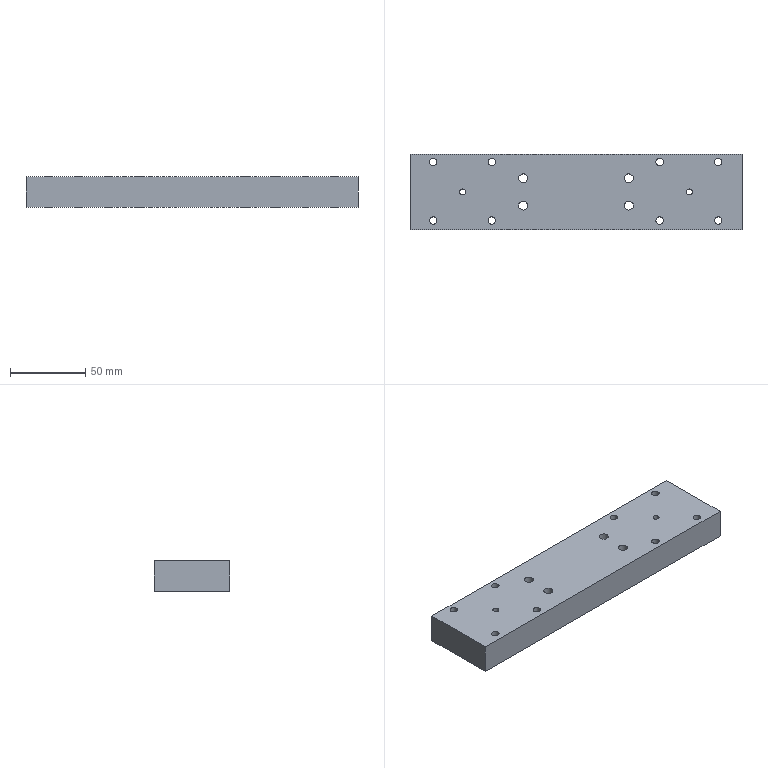NC program | NX | posted with a generic post | part box 220 x 50 x 20 mm
Whole program:
N10 G17 G21 G94 G90
(ZLEVEL_PROFILE_1 , TOOL : D10)
N12 T10 M6
N14 G54
N16 G17 G0 G90 X-42.544 Y30.1 S9500 M3
N18 G43 Z30. H10
N20 Z1.5
N22 G94 G1 X0. Z-0.73 F3000.
N24 X110.
N26 G2 X115.1 Y25. R5.1
N28 G1 Y-25.
N30 G2 X110. Y-30.1 R5.1
N32 G1 X-110.
N34 G2 X-115.1 Y-25. R5.1
N36 G1 Y25.
N38 G2 X-110. Y30.1 R5.1
N40 G1 X0.
N42 X41.8 Z-1.459
N44 X110.
N46 G2 X115.1 Y25. R5.1
N48 G1 Y-25.
N50 G2 X110. Y-30.1 R5.1
N52 G1 X-110.
N54 G2 X-115.1 Y-25. R5.1
N56 G1 Y25.
N58 G2 X-110. Y30.1 R5.1
N60 G1 X0.
N62 X41.8 Z-2.189
N64 X110.
N66 G2 X115.1 Y25. R5.1
N68 G1 Y-25.
N70 G2 X110. Y-30.1 R5.1
N72 G1 X-110.
N74 G2 X-115.1 Y-25. R5.1
N76 G1 Y25.
N78 G2 X-110. Y30.1 R5.1
N80 G1 X0.
N82 X41.8 Z-2.919
N84 X110.
N86 G2 X115.1 Y25. R5.1
N88 G1 Y-25.
N90 G2 X110. Y-30.1 R5.1
N92 G1 X-110.
N94 G2 X-115.1 Y-25. R5.1
N96 G1 Y25.
N98 G2 X-110. Y30.1 R5.1
N100 G1 X0.
N102 X41.8 Z-3.648
N104 X110.
N106 G2 X115.1 Y25. R5.1
N108 G1 Y-25.
N110 G2 X110. Y-30.1 R5.1
N112 G1 X-110.
N114 G2 X-115.1 Y-25. R5.1
N116 G1 Y25.
N118 G2 X-110. Y30.1 R5.1
N120 G1 X0.
N122 X41.8 Z-4.378
N124 X110.
N126 G2 X115.1 Y25. R5.1
N128 G1 Y-25.
N130 G2 X110. Y-30.1 R5.1
N132 G1 X-110.
N134 G2 X-115.1 Y-25. R5.1
N136 G1 Y25.
N138 G2 X-110. Y30.1 R5.1
N140 G1 X0.
N142 X41.8 Z-5.107
N144 X110.
N146 G2 X115.1 Y25. R5.1
N148 G1 Y-25.
N150 G2 X110. Y-30.1 R5.1
N152 G1 X-110.
N154 G2 X-115.1 Y-25. R5.1
N156 G1 Y25.
N158 G2 X-110. Y30.1 R5.1
N160 G1 X0.
N162 X41.8 Z-5.837
N164 X110.
N166 G2 X115.1 Y25. R5.1
N168 G1 Y-25.
N170 G2 X110. Y-30.1 R5.1
N172 G1 X-110.
N174 G2 X-115.1 Y-25. R5.1
N176 G1 Y25.
N178 G2 X-110. Y30.1 R5.1
N180 G1 X0.
N182 X41.8 Z-6.567
N184 X110.
N186 G2 X115.1 Y25. R5.1
N188 G1 Y-25.
N190 G2 X110. Y-30.1 R5.1
N192 G1 X-110.
N194 G2 X-115.1 Y-25. R5.1
N196 G1 Y25.
N198 G2 X-110. Y30.1 R5.1
N200 G1 X0.
N202 X41.8 Z-7.296
N204 X110.
N206 G2 X115.1 Y25. R5.1
N208 G1 Y-25.
N210 G2 X110. Y-30.1 R5.1
N212 G1 X-110.
N214 G2 X-115.1 Y-25. R5.1
N216 G1 Y25.
N218 G2 X-110. Y30.1 R5.1
N220 G1 X0.
N222 X41.8 Z-8.026
N224 X110.
N226 G2 X115.1 Y25. R5.1
N228 G1 Y-25.
N230 G2 X110. Y-30.1 R5.1
N232 G1 X-110.
N234 G2 X-115.1 Y-25. R5.1
N236 G1 Y25.
N238 G2 X-110. Y30.1 R5.1
N240 G1 X0.
N242 X41.8 Z-8.756
N244 X110.
N246 G2 X115.1 Y25. R5.1
N248 G1 Y-25.
N250 G2 X110. Y-30.1 R5.1
N252 G1 X-110.
N254 G2 X-115.1 Y-25. R5.1
N256 G1 Y25.
N258 G2 X-110. Y30.1 R5.1
N260 G1 X0.
N262 X41.8 Z-9.485
N264 X110.
N266 G2 X115.1 Y25. R5.1
N268 G1 Y-25.
N270 G2 X110. Y-30.1 R5.1
N272 G1 X-110.
N274 G2 X-115.1 Y-25. R5.1
N276 G1 Y25.
N278 G2 X-110. Y30.1 R5.1
N280 G1 X0.
N282 X41.8 Z-10.215
N284 X110.
N286 G2 X115.1 Y25. R5.1
N288 G1 Y-25.
N290 G2 X110. Y-30.1 R5.1
N292 G1 X-110.
N294 G2 X-115.1 Y-25. R5.1
N296 G1 Y25.
N298 G2 X-110. Y30.1 R5.1
N300 G1 X0.
N302 X41.8 Z-10.944
N304 X110.
N306 G2 X115.1 Y25. R5.1
N308 G1 Y-25.
N310 G2 X110. Y-30.1 R5.1
N312 G1 X-110.
N314 G2 X-115.1 Y-25. R5.1
N316 G1 Y25.
N318 G2 X-110. Y30.1 R5.1
N320 G1 X0.
N322 X41.8 Z-11.674
N324 X110.
N326 G2 X115.1 Y25. R5.1
N328 G1 Y-25.
N330 G2 X110. Y-30.1 R5.1
N332 G1 X-110.
N334 G2 X-115.1 Y-25. R5.1
N336 G1 Y25.
N338 G2 X-110. Y30.1 R5.1
N340 G1 X0.
N342 X41.8 Z-12.404
N344 X110.
N346 G2 X115.1 Y25. R5.1
N348 G1 Y-25.
N350 G2 X110. Y-30.1 R5.1
N352 G1 X-110.
N354 G2 X-115.1 Y-25. R5.1
N356 G1 Y25.
N358 G2 X-110. Y30.1 R5.1
N360 G1 X0.
N362 X41.8 Z-13.133
N364 X110.
N366 G2 X115.1 Y25. R5.1
N368 G1 Y-25.
N370 G2 X110. Y-30.1 R5.1
N372 G1 X-110.
N374 G2 X-115.1 Y-25. R5.1
N376 G1 Y25.
N378 G2 X-110. Y30.1 R5.1
N380 G1 X0.
N382 X41.8 Z-13.863
N384 X110.
N386 G2 X115.1 Y25. R5.1
N388 G1 Y-25.
N390 G2 X110. Y-30.1 R5.1
N392 G1 X-110.
N394 G2 X-115.1 Y-25. R5.1
N396 G1 Y25.
N398 G2 X-110. Y30.1 R5.1
N400 G1 X0.
N402 X41.8 Z-14.593
N404 X110.
N406 G2 X115.1 Y25. R5.1
N408 G1 Y-25.
N410 G2 X110. Y-30.1 R5.1
N412 G1 X-110.
N414 G2 X-115.1 Y-25. R5.1
N416 G1 Y25.
N418 G2 X-110. Y30.1 R5.1
N420 G1 X0.
N422 X41.8 Z-15.322
N424 X110.
N426 G2 X115.1 Y25. R5.1
N428 G1 Y-25.
N430 G2 X110. Y-30.1 R5.1
N432 G1 X-110.
N434 G2 X-115.1 Y-25. R5.1
N436 G1 Y25.
N438 G2 X-110. Y30.1 R5.1
N440 G1 X0.
N442 X41.8 Z-16.052
N444 X110.
N446 G2 X115.1 Y25. R5.1
N448 G1 Y-25.
N450 G2 X110. Y-30.1 R5.1
N452 G1 X-110.
N454 G2 X-115.1 Y-25. R5.1
N456 G1 Y25.
N458 G2 X-110. Y30.1 R5.1
N460 G1 X0.
N462 X41.8 Z-16.781
N464 X110.
N466 G2 X115.1 Y25. R5.1
N468 G1 Y-25.
N470 G2 X110. Y-30.1 R5.1
N472 G1 X-110.
N474 G2 X-115.1 Y-25. R5.1
N476 G1 Y25.
N478 G2 X-110. Y30.1 R5.1
N480 G1 X0.
N482 X41.8 Z-17.511
N484 X110.
N486 G2 X115.1 Y25. R5.1
N488 G1 Y-25.
N490 G2 X110. Y-30.1 R5.1
N492 G1 X-110.
N494 G2 X-115.1 Y-25. R5.1
N496 G1 Y25.
N498 G2 X-110. Y30.1 R5.1
N500 G1 X0.
N502 X41.8 Z-18.241
N504 X110.
N506 G2 X115.1 Y25. R5.1
N508 G1 Y-25.
N510 G2 X110. Y-30.1 R5.1
N512 G1 X-110.
N514 G2 X-115.1 Y-25. R5.1
N516 G1 Y25.
N518 G2 X-110. Y30.1 R5.1
N520 G1 X0.
N522 X41.8 Z-18.97
N524 X110.
N526 G2 X115.1 Y25. R5.1
N528 G1 Y-25.
N530 G2 X110. Y-30.1 R5.1
N532 G1 X-110.
N534 G2 X-115.1 Y-25. R5.1
N536 G1 Y25.
N538 G2 X-110. Y30.1 R5.1
N540 G1 X0.
N542 X41.8 Z-19.7
N544 X110.
N546 G2 X115.1 Y25. R5.1
N548 G1 Y-25.
N550 G2 X110. Y-30.1 R5.1
N552 G1 X-110.
N554 G2 X-115.1 Y-25. R5.1
N556 G1 Y25.
N558 G2 X-110. Y30.1 R5.1
N560 G1 X41.8
N562 Z-18.2
N564 G0 Z30.
N566 M5
(ZLEVEL_PROFILE , TOOL : D10JING)
N568 T11 M6
N570 G54
N572 G17 G0 G90 X-111.622 Y31.809 S9500 M3
N574 G43 Z30. H11
N576 Z-18.3
N578 G94 G1 Z-19.8 F1250.
N580 X-110.866 Y30.5
N582 G3 X-110. Y30. R1.
N584 G1 X110.
N586 G2 X115. Y25. R5.
N588 G1 Y-25.
N590 G2 X110. Y-30. R5.
N592 G1 X-110.
N594 G2 X-115. Y-25. R5.
N596 G1 Y25.
N598 G2 X-110. Y30. R5.
N600 G3 X-109.134 Y30.5 R1.
N602 G1 X-108.268 Y32.
N604 Z-18.3
N606 G0 Z30.
N608 M5
(PLANAR_MILL , TOOL : D6A45)
N610 T07 M6
N612 G54
N614 G17 G0 G90 X93.389 Y-20.287 S9500 M3
N616 G43 Z30. H7
N618 Z2.
N620 G94 G1 Z-1. F500.
N622 G3 X94.255 Y-20.787 R1.
N624 X96.055 Y-18.987 R1.8 F1250.
N626 X94.255 Y-20.787 R-1.8
N628 X95.121 Y-20.287 R1.
N630 G1 Z2.
N632 G0 Z30.
N634 X74.134 Y-0.8
N636 Z2.
N638 G1 Z-1. F500.
N640 G3 X75. Y-1.3 R1.
N642 X76.3 Y0. R1.3 F1250.
N644 X75. Y-1.3 R-1.3
N646 X75.866 Y-0.8 R1.
N648 G1 Z2.
N650 G0 Z30.
N652 X95.121 Y21.204
N654 Z2.
N656 G1 Z-1. F500.
N658 G3 X94.255 Y21.704 R1.
N660 X92.455 Y19.904 R1.8 F1250.
N662 X94.255 Y21.704 R-1.8
N664 X93.389 Y21.204 R1.
N666 G1 Z2.
N668 G0 Z30.
N670 X56.231
N672 Z2.
N674 G1 Z-1. F500.
N676 G3 X55.365 Y21.704 R1.
N678 X53.565 Y19.904 R1.8 F1250.
N680 X55.365 Y21.704 R-1.8
N682 X54.499 Y21.204 R1.
N684 G1 Z2.
N686 G0 Z30.
N688 X35.866 Y10.8
N690 Z2.
N692 G1 Z-1. F500.
N694 G3 X35. Y11.3 R1.
N696 X32.7 Y9. R2.3 F1250.
N698 X35. Y11.3 R-2.3
N700 X34.134 Y10.8 R1.
N702 G1 Z2.
N704 G0 Z30.
N706 X54.499 Y-20.287
N708 Z2.
N710 G1 Z-1. F500.
N712 G3 X55.365 Y-20.787 R1.
N714 X57.165 Y-18.987 R1.8 F1250.
N716 X55.365 Y-20.787 R-1.8
N718 X56.231 Y-20.287 R1.
N720 G1 Z2.
N722 G0 Z30.
N724 X34.134 Y-10.8
N726 Z2.
N728 G1 Z-1. F500.
N730 G3 X35. Y-11.3 R1.
N732 X37.3 Y-9. R2.3 F1250.
N734 X35. Y-11.3 R-2.3
N736 X35.866 Y-10.8 R1.
N738 G1 Z2.
N740 G0 Z30.
N742 X0.866 Y-26.2
N744 Z2.
N746 G1 Z-1. F500.
N748 G3 X0. Y-25.7 R1.
N750 G1 X-110. F1250.
N752 G2 X-110.7 Y-25. R0.7
N754 G1 Y25.
N756 G2 X-110. Y25.7 R0.7
N758 G1 X110.
N760 G2 X110.7 Y25. R0.7
N762 G1 Y-25.
N764 G2 X110. Y-25.7 R0.7
N766 G1 X0.
N768 G3 X-0.866 Y-26.2 R1.
N770 G1 Z2.
N772 G0 Z30.
N774 X-35.866 Y-10.8
N776 Z2.
N778 G1 Z-1. F500.
N780 G3 X-35. Y-11.3 R1.
N782 X-32.7 Y-9. R2.3 F1250.
N784 X-35. Y-11.3 R-2.3
N786 X-34.134 Y-10.8 R1.
N788 G1 Z2.
N790 G0 Z30.
N792 X-56.611 Y-20.287
N794 Z2.
N796 G1 Z-1. F500.
N798 G3 X-55.745 Y-20.787 R1.
N800 X-53.945 Y-18.987 R1.8 F1250.
N802 X-55.745 Y-20.787 R-1.8
N804 X-54.879 Y-20.287 R1.
N806 G1 Z2.
N808 G0 Z30.
N810 X-34.134 Y10.8
N812 Z2.
N814 G1 Z-1. F500.
N816 G3 X-35. Y11.3 R1.
N818 X-37.3 Y9. R2.3 F1250.
N820 X-35. Y11.3 R-2.3
N822 X-35.866 Y10.8 R1.
N824 G1 Z2.
N826 G0 Z30.
N828 X-54.879 Y21.204
N830 Z2.
N832 G1 Z-1. F500.
N834 G3 X-55.745 Y21.704 R1.
N836 X-57.545 Y19.904 R1.8 F1250.
N838 X-55.745 Y21.704 R-1.8
N840 X-56.611 Y21.204 R1.
N842 G1 Z2.
N844 G0 Z30.
N846 X-74.134 Y0.8
N848 Z2.
N850 G1 Z-1. F500.
N852 G3 X-75. Y1.3 R1.
N854 X-76.3 Y0. R1.3 F1250.
N856 X-75. Y1.3 R-1.3
N858 X-75.866 Y0.8 R1.
N860 G1 Z2.
N862 G0 Z30.
N864 X-95.501 Y-20.287
N866 Z2.
N868 G1 Z-1. F500.
N870 G3 X-94.635 Y-20.787 R1.
N872 X-92.835 Y-18.987 R1.8 F1250.
N874 X-94.635 Y-20.787 R-1.8
N876 X-93.769 Y-20.287 R1.
N878 G1 Z2.
N880 G0 Z30.
N882 Y21.204
N884 Z2.
N886 G1 Z-1. F500.
N888 G3 X-94.635 Y21.704 R1.
N890 X-96.435 Y19.904 R1.8 F1250.
N892 X-94.635 Y21.704 R-1.8
N894 X-95.501 Y21.204 R1.
N896 G1 Z2.
N898 G0 Z30.
N900 M5
N902 M2